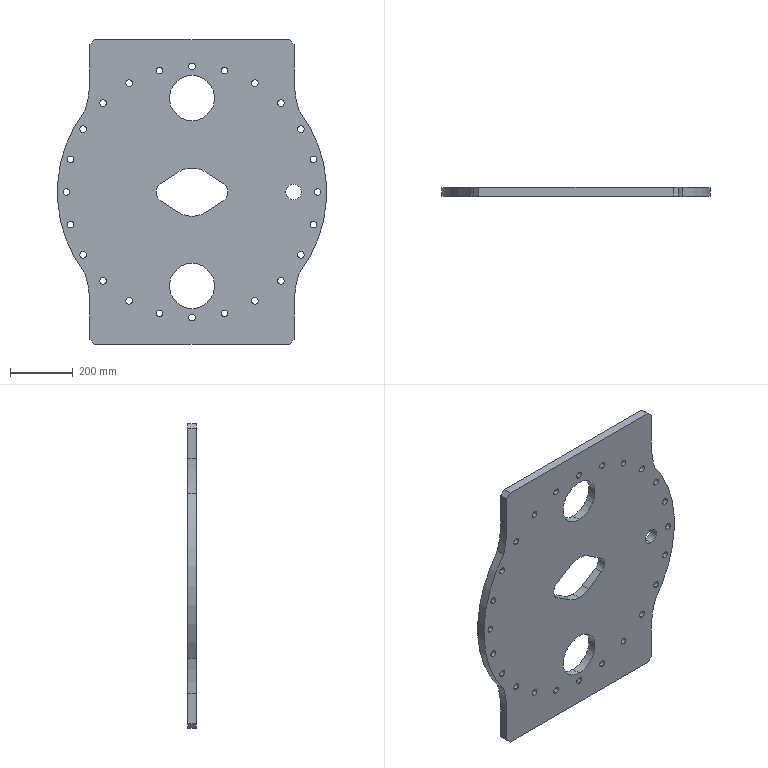Part | SolidWorks | features Extrusion 1, ICE 1 | 1 solid | 81 faces | box 857 x 28 x 970 mm | volume 18025992 mm3 | cylinder 65 | plane 16 | commonest cylinder face diameters 21 x48 144 x4 706 x4 154.726 x3 50 x2 63.719 x2